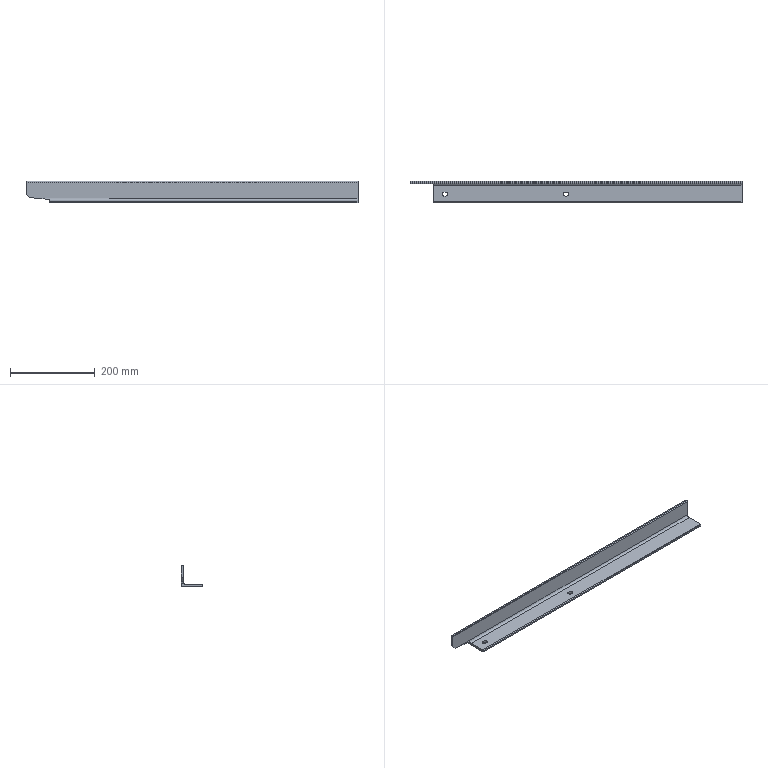Part | SolidWorks | 1 solid | 25 faces | box 783.5 x 50 x 50 mm | volume 359251 mm3 | plane 16 | cylinder 9 | commonest cylinder face diameters 9 x6 3.333 x2 11 x1
STEP:
#1=CARTESIAN_POINT('',(-21.75,-25.5,0.));
#2=VERTEX_POINT('',#1);
#3=CARTESIAN_POINT('',(-17.25,-30.,0.));
#4=VERTEX_POINT('',#3);
#5=CARTESIAN_POINT('',(-21.75,-30.,0.));
#6=DIRECTION('',(0.,0.,-1.));
#7=DIRECTION('',(1.,0.,0.));
#8=AXIS2_PLACEMENT_3D('',#5,#6,#7);
#9=CIRCLE('',#8,4.5);
#10=EDGE_CURVE('',#2,#4,#9,.T.);
#11=ORIENTED_EDGE('',*,*,#10,.T.);
#12=CARTESIAN_POINT('',(-17.25,-30.,5.));
#13=VERTEX_POINT('',#12);
#14=CARTESIAN_POINT('',(-17.25,-30.,-0.001));
#15=DIRECTION('',(0.,0.,1.));
#16=VECTOR('',#15,1000.);
#17=LINE('',#14,#16);
#18=EDGE_CURVE('',#4,#13,#17,.T.);
#19=ORIENTED_EDGE('',*,*,#18,.T.);
#20=CARTESIAN_POINT('',(-21.75,-25.5,5.));
#21=VERTEX_POINT('',#20);
#22=CARTESIAN_POINT('',(-21.75,-30.,5.));
#23=DIRECTION('',(0.,0.,1.));
#24=DIRECTION('',(1.,0.,0.));
#25=AXIS2_PLACEMENT_3D('',#22,#23,#24);
#26=CIRCLE('',#25,4.5);
#27=EDGE_CURVE('',#13,#21,#26,.T.);
#28=ORIENTED_EDGE('',*,*,#27,.T.);
#29=CARTESIAN_POINT('',(-21.75,-25.5,-0.001));
#30=DIRECTION('',(0.,0.,1.));
#31=VECTOR('',#30,1000.);
#32=LINE('',#29,#31);
#33=EDGE_CURVE('',#2,#21,#32,.T.);
#34=ORIENTED_EDGE('',*,*,#33,.F.);
#35=EDGE_LOOP('',(#11,#19,#28,#34));
#36=FACE_OUTER_BOUND('',#35,.T.);
#37=CARTESIAN_POINT('',(-21.75,-30.,-0.001));
#38=DIRECTION('',(0.,0.,1.));
#39=DIRECTION('',(1.,0.,0.));
#40=AXIS2_PLACEMENT_3D('',#37,#38,#39);
#41=CYLINDRICAL_SURFACE('',#40,4.5);
#42=ADVANCED_FACE('',(#36),#41,.F.);
#43=CARTESIAN_POINT('',(-307.75,-25.5,0.));
#44=VERTEX_POINT('',#43);
#45=CARTESIAN_POINT('',(-303.25,-30.,0.));
#46=VERTEX_POINT('',#45);
#47=CARTESIAN_POINT('',(-307.75,-30.,0.));
#48=DIRECTION('',(0.,0.,-1.));
#49=DIRECTION('',(1.,0.,0.));
#50=AXIS2_PLACEMENT_3D('',#47,#48,#49);
#51=CIRCLE('',#50,4.5);
#52=EDGE_CURVE('',#44,#46,#51,.T.);
#53=ORIENTED_EDGE('',*,*,#52,.T.);
#54=CARTESIAN_POINT('',(-303.25,-30.,5.));
#55=VERTEX_POINT('',#54);
#56=CARTESIAN_POINT('',(-303.25,-30.,-0.001));
#57=DIRECTION('',(0.,0.,1.));
#58=VECTOR('',#57,1000.);
#59=LINE('',#56,#58);
#60=EDGE_CURVE('',#46,#55,#59,.T.);
#61=ORIENTED_EDGE('',*,*,#60,.T.);
#62=CARTESIAN_POINT('',(-307.75,-25.5,5.));
#63=VERTEX_POINT('',#62);
#64=CARTESIAN_POINT('',(-307.75,-30.,5.));
#65=DIRECTION('',(0.,0.,1.));
#66=DIRECTION('',(1.,0.,0.));
#67=AXIS2_PLACEMENT_3D('',#64,#65,#66);
#68=CIRCLE('',#67,4.5);
#69=EDGE_CURVE('',#55,#63,#68,.T.);
#70=ORIENTED_EDGE('',*,*,#69,.T.);
#71=CARTESIAN_POINT('',(-307.75,-25.5,-0.001));
#72=DIRECTION('',(0.,0.,1.));
#73=VECTOR('',#72,1000.);
#74=LINE('',#71,#73);
#75=EDGE_CURVE('',#44,#63,#74,.T.);
#76=ORIENTED_EDGE('',*,*,#75,.F.);
#77=EDGE_LOOP('',(#53,#61,#70,#76));
#78=FACE_OUTER_BOUND('',#77,.T.);
#79=CARTESIAN_POINT('',(-307.75,-30.,-0.001));
#80=DIRECTION('',(0.,0.,1.));
#81=DIRECTION('',(1.,0.,0.));
#82=AXIS2_PLACEMENT_3D('',#79,#80,#81);
#83=CYLINDRICAL_SURFACE('',#82,4.5);
#84=ADVANCED_FACE('',(#78),#83,.F.);
#85=CARTESIAN_POINT('',(-25.75,-25.5,0.));
#86=VERTEX_POINT('',#85);
#87=CARTESIAN_POINT('',(-25.75,-25.5,0.));
#88=DIRECTION('',(1.,0.,0.));
#89=VECTOR('',#88,1000.);
#90=LINE('',#87,#89);
#91=EDGE_CURVE('',#86,#2,#90,.T.);
#92=ORIENTED_EDGE('',*,*,#91,.F.);
#93=CARTESIAN_POINT('',(-25.75,-34.5,0.));
#94=VERTEX_POINT('',#93);
#95=CARTESIAN_POINT('',(-25.75,-30.,0.));
#96=DIRECTION('',(0.,0.,-1.));
#97=DIRECTION('',(1.,0.,0.));
#98=AXIS2_PLACEMENT_3D('',#95,#96,#97);
#99=CIRCLE('',#98,4.5);
#100=EDGE_CURVE('',#94,#86,#99,.T.);
#101=ORIENTED_EDGE('',*,*,#100,.F.);
#102=CARTESIAN_POINT('',(-21.75,-34.5,0.));
#103=VERTEX_POINT('',#102);
#104=CARTESIAN_POINT('',(-25.75,-34.5,0.));
#105=DIRECTION('',(-1.,0.,0.));
#106=VECTOR('',#105,1000.);
#107=LINE('',#104,#106);
#108=EDGE_CURVE('',#103,#94,#107,.T.);
#109=ORIENTED_EDGE('',*,*,#108,.F.);
#110=CARTESIAN_POINT('',(-21.75,-30.,0.));
#111=DIRECTION('',(0.,0.,-1.));
#112=DIRECTION('',(1.,0.,0.));
#113=AXIS2_PLACEMENT_3D('',#110,#111,#112);
#114=CIRCLE('',#113,4.5);
#115=EDGE_CURVE('',#4,#103,#114,.T.);
#116=ORIENTED_EDGE('',*,*,#115,.F.);
#117=ORIENTED_EDGE('',*,*,#10,.F.);
#118=EDGE_LOOP('',(#92,#101,#109,#116,#117));
#119=FACE_BOUND('',#118,.T.);
#120=CARTESIAN_POINT('',(-311.75,-25.5,0.));
#121=VERTEX_POINT('',#120);
#122=CARTESIAN_POINT('',(-311.75,-25.5,0.));
#123=DIRECTION('',(1.,0.,0.));
#124=VECTOR('',#123,1000.);
#125=LINE('',#122,#124);
#126=EDGE_CURVE('',#121,#44,#125,.T.);
#127=ORIENTED_EDGE('',*,*,#126,.F.);
#128=CARTESIAN_POINT('',(-311.75,-34.5,0.));
#129=VERTEX_POINT('',#128);
#130=CARTESIAN_POINT('',(-311.75,-30.,0.));
#131=DIRECTION('',(0.,0.,-1.));
#132=DIRECTION('',(1.,0.,0.));
#133=AXIS2_PLACEMENT_3D('',#130,#131,#132);
#134=CIRCLE('',#133,4.5);
#135=EDGE_CURVE('',#129,#121,#134,.T.);
#136=ORIENTED_EDGE('',*,*,#135,.F.);
#137=CARTESIAN_POINT('',(-307.75,-34.5,0.));
#138=VERTEX_POINT('',#137);
#139=CARTESIAN_POINT('',(-311.75,-34.5,0.));
#140=DIRECTION('',(-1.,0.,0.));
#141=VECTOR('',#140,1000.);
#142=LINE('',#139,#141);
#143=EDGE_CURVE('',#138,#129,#142,.T.);
#144=ORIENTED_EDGE('',*,*,#143,.F.);
#145=CARTESIAN_POINT('',(-307.75,-30.,0.));
#146=DIRECTION('',(0.,0.,-1.));
#147=DIRECTION('',(1.,0.,0.));
#148=AXIS2_PLACEMENT_3D('',#145,#146,#147);
#149=CIRCLE('',#148,4.5);
#150=EDGE_CURVE('',#46,#138,#149,.T.);
#151=ORIENTED_EDGE('',*,*,#150,.F.);
#152=ORIENTED_EDGE('',*,*,#52,.F.);
#153=EDGE_LOOP('',(#127,#136,#144,#151,#152));
#154=FACE_BOUND('',#153,.T.);
#155=CARTESIAN_POINT('',(-335.25,-50.,0.));
#156=VERTEX_POINT('',#155);
#157=CARTESIAN_POINT('',(391.75,-50.,0.));
#158=VERTEX_POINT('',#157);
#159=CARTESIAN_POINT('',(-391.75,-50.,0.));
#160=DIRECTION('',(1.,0.,0.));
#161=VECTOR('',#160,1000.);
#162=LINE('',#159,#161);
#163=EDGE_CURVE('',#156,#158,#162,.T.);
#164=ORIENTED_EDGE('',*,*,#163,.F.);
#165=CARTESIAN_POINT('',(-335.25,0.,0.));
#166=VERTEX_POINT('',#165);
#167=CARTESIAN_POINT('',(-335.25,-50.,0.));
#168=DIRECTION('',(0.,1.,0.));
#169=VECTOR('',#168,1000.);
#170=LINE('',#167,#169);
#171=EDGE_CURVE('',#156,#166,#170,.T.);
#172=ORIENTED_EDGE('',*,*,#171,.T.);
#173=CARTESIAN_POINT('',(391.75,0.,0.));
#174=VERTEX_POINT('',#173);
#175=CARTESIAN_POINT('',(-391.75,0.,0.));
#176=DIRECTION('',(1.,0.,0.));
#177=VECTOR('',#176,1000.);
#178=LINE('',#175,#177);
#179=EDGE_CURVE('',#166,#174,#178,.T.);
#180=ORIENTED_EDGE('',*,*,#179,.T.);
#181=CARTESIAN_POINT('',(391.75,-50.,0.));
#182=DIRECTION('',(0.,-1.,0.));
#183=VECTOR('',#182,1000.);
#184=LINE('',#181,#183);
#185=EDGE_CURVE('',#174,#158,#184,.T.);
#186=ORIENTED_EDGE('',*,*,#185,.T.);
#187=EDGE_LOOP('',(#164,#172,#180,#186));
#188=FACE_OUTER_BOUND('',#187,.T.);
#189=CARTESIAN_POINT('',(-391.75,-50.,0.));
#190=DIRECTION('',(0.,0.,1.));
#191=DIRECTION('',(1.,0.,0.));
#192=AXIS2_PLACEMENT_3D('',#189,#190,#191);
#193=PLANE('',#192);
#194=ADVANCED_FACE('',(#119,#154,#188),#193,.F.);
#195=CARTESIAN_POINT('',(-335.25,-50.,3.333));
#196=VERTEX_POINT('',#195);
#197=CARTESIAN_POINT('',(391.75,-50.,3.333));
#198=VERTEX_POINT('',#197);
#199=CARTESIAN_POINT('',(-391.75,-50.,3.333));
#200=DIRECTION('',(1.,0.,0.));
#201=VECTOR('',#200,1000.);
#202=LINE('',#199,#201);
#203=EDGE_CURVE('',#196,#198,#202,.T.);
#204=ORIENTED_EDGE('',*,*,#203,.F.);
#205=CARTESIAN_POINT('',(-335.25,-50.,-7.499));
#206=DIRECTION('',(0.,0.,-1.));
#207=VECTOR('',#206,1000.);
#208=LINE('',#205,#207);
#209=EDGE_CURVE('',#196,#156,#208,.T.);
#210=ORIENTED_EDGE('',*,*,#209,.T.);
#211=ORIENTED_EDGE('',*,*,#163,.T.);
#212=CARTESIAN_POINT('',(391.75,-50.,0.));
#213=DIRECTION('',(0.,0.,1.));
#214=VECTOR('',#213,1000.);
#215=LINE('',#212,#214);
#216=EDGE_CURVE('',#158,#198,#215,.T.);
#217=ORIENTED_EDGE('',*,*,#216,.T.);
#218=EDGE_LOOP('',(#204,#210,#211,#217));
#219=FACE_OUTER_BOUND('',#218,.T.);
#220=CARTESIAN_POINT('',(-391.75,-50.,0.));
#221=DIRECTION('',(0.,1.,0.));
#222=DIRECTION('',(-1.,0.,0.));
#223=AXIS2_PLACEMENT_3D('',#220,#221,#222);
#224=PLANE('',#223);
#225=ADVANCED_FACE('',(#219),#224,.F.);
#226=CARTESIAN_POINT('',(-335.25,-48.333,5.));
#227=VERTEX_POINT('',#226);
#228=CARTESIAN_POINT('',(391.75,-48.333,5.));
#229=VERTEX_POINT('',#228);
#230=CARTESIAN_POINT('',(-391.75,-48.333,5.));
#231=DIRECTION('',(1.,0.,0.));
#232=VECTOR('',#231,1000.);
#233=LINE('',#230,#232);
#234=EDGE_CURVE('',#227,#229,#233,.T.);
#235=ORIENTED_EDGE('',*,*,#234,.F.);
#236=CARTESIAN_POINT('',(-335.25,-48.333,3.333));
#237=DIRECTION('',(1.,0.,0.));
#238=DIRECTION('',(0.,0.,-1.));
#239=AXIS2_PLACEMENT_3D('',#236,#237,#238);
#240=CIRCLE('',#239,1.667);
#241=EDGE_CURVE('',#227,#196,#240,.T.);
#242=ORIENTED_EDGE('',*,*,#241,.T.);
#243=ORIENTED_EDGE('',*,*,#203,.T.);
#244=CARTESIAN_POINT('',(391.75,-48.333,3.333));
#245=DIRECTION('',(-1.,0.,0.));
#246=DIRECTION('',(0.,-1.,0.));
#247=AXIS2_PLACEMENT_3D('',#244,#245,#246);
#248=CIRCLE('',#247,1.667);
#249=EDGE_CURVE('',#198,#229,#248,.T.);
#250=ORIENTED_EDGE('',*,*,#249,.T.);
#251=EDGE_LOOP('',(#235,#242,#243,#250));
#252=FACE_OUTER_BOUND('',#251,.T.);
#253=CARTESIAN_POINT('',(-391.75,-48.333,3.333));
#254=DIRECTION('',(1.,0.,0.));
#255=DIRECTION('',(0.,1.,0.));
#256=AXIS2_PLACEMENT_3D('',#253,#254,#255);
#257=CYLINDRICAL_SURFACE('',#256,1.667);
#258=ADVANCED_FACE('',(#252),#257,.T.);
#259=CARTESIAN_POINT('',(-25.75,-34.5,5.));
#260=VERTEX_POINT('',#259);
#261=CARTESIAN_POINT('',(-21.75,-34.5,5.));
#262=VERTEX_POINT('',#261);
#263=CARTESIAN_POINT('',(-25.75,-34.5,5.));
#264=DIRECTION('',(1.,0.,0.));
#265=VECTOR('',#264,1000.);
#266=LINE('',#263,#265);
#267=EDGE_CURVE('',#260,#262,#266,.T.);
#268=ORIENTED_EDGE('',*,*,#267,.F.);
#269=CARTESIAN_POINT('',(-25.75,-25.5,5.));
#270=VERTEX_POINT('',#269);
#271=CARTESIAN_POINT('',(-25.75,-30.,5.));
#272=DIRECTION('',(0.,0.,1.));
#273=DIRECTION('',(1.,0.,0.));
#274=AXIS2_PLACEMENT_3D('',#271,#272,#273);
#275=CIRCLE('',#274,4.5);
#276=EDGE_CURVE('',#270,#260,#275,.T.);
#277=ORIENTED_EDGE('',*,*,#276,.F.);
#278=CARTESIAN_POINT('',(-25.75,-25.5,5.));
#279=DIRECTION('',(-1.,0.,0.));
#280=VECTOR('',#279,1000.);
#281=LINE('',#278,#280);
#282=EDGE_CURVE('',#21,#270,#281,.T.);
#283=ORIENTED_EDGE('',*,*,#282,.F.);
#284=ORIENTED_EDGE('',*,*,#27,.F.);
#285=CARTESIAN_POINT('',(-21.75,-30.,5.));
#286=DIRECTION('',(0.,0.,1.));
#287=DIRECTION('',(1.,0.,0.));
#288=AXIS2_PLACEMENT_3D('',#285,#286,#287);
#289=CIRCLE('',#288,4.5);
#290=EDGE_CURVE('',#262,#13,#289,.T.);
#291=ORIENTED_EDGE('',*,*,#290,.F.);
#292=EDGE_LOOP('',(#268,#277,#283,#284,#291));
#293=FACE_BOUND('',#292,.T.);
#294=CARTESIAN_POINT('',(-311.75,-34.5,5.));
#295=VERTEX_POINT('',#294);
#296=CARTESIAN_POINT('',(-307.75,-34.5,5.));
#297=VERTEX_POINT('',#296);
#298=CARTESIAN_POINT('',(-311.75,-34.5,5.));
#299=DIRECTION('',(1.,0.,0.));
#300=VECTOR('',#299,1000.);
#301=LINE('',#298,#300);
#302=EDGE_CURVE('',#295,#297,#301,.T.);
#303=ORIENTED_EDGE('',*,*,#302,.F.);
#304=CARTESIAN_POINT('',(-311.75,-25.5,5.));
#305=VERTEX_POINT('',#304);
#306=CARTESIAN_POINT('',(-311.75,-30.,5.));
#307=DIRECTION('',(0.,0.,1.));
#308=DIRECTION('',(1.,0.,0.));
#309=AXIS2_PLACEMENT_3D('',#306,#307,#308);
#310=CIRCLE('',#309,4.5);
#311=EDGE_CURVE('',#305,#295,#310,.T.);
#312=ORIENTED_EDGE('',*,*,#311,.F.);
#313=CARTESIAN_POINT('',(-311.75,-25.5,5.));
#314=DIRECTION('',(-1.,0.,0.));
#315=VECTOR('',#314,1000.);
#316=LINE('',#313,#315);
#317=EDGE_CURVE('',#63,#305,#316,.T.);
#318=ORIENTED_EDGE('',*,*,#317,.F.);
#319=ORIENTED_EDGE('',*,*,#69,.F.);
#320=CARTESIAN_POINT('',(-307.75,-30.,5.));
#321=DIRECTION('',(0.,0.,1.));
#322=DIRECTION('',(1.,0.,0.));
#323=AXIS2_PLACEMENT_3D('',#320,#321,#322);
#324=CIRCLE('',#323,4.5);
#325=EDGE_CURVE('',#297,#55,#324,.T.);
#326=ORIENTED_EDGE('',*,*,#325,.F.);
#327=EDGE_LOOP('',(#303,#312,#318,#319,#326));
#328=FACE_BOUND('',#327,.T.);
#329=CARTESIAN_POINT('',(-335.25,-10.5,5.));
#330=VERTEX_POINT('',#329);
#331=CARTESIAN_POINT('',(391.75,-10.5,5.));
#332=VERTEX_POINT('',#331);
#333=CARTESIAN_POINT('',(-391.75,-10.5,5.));
#334=DIRECTION('',(1.,0.,0.));
#335=VECTOR('',#334,1000.);
#336=LINE('',#333,#335);
#337=EDGE_CURVE('',#330,#332,#336,.T.);
#338=ORIENTED_EDGE('',*,*,#337,.F.);
#339=CARTESIAN_POINT('',(-335.25,-10.5,5.));
#340=DIRECTION('',(0.,-1.,0.));
#341=VECTOR('',#340,1000.);
#342=LINE('',#339,#341);
#343=EDGE_CURVE('',#330,#227,#342,.T.);
#344=ORIENTED_EDGE('',*,*,#343,.T.);
#345=ORIENTED_EDGE('',*,*,#234,.T.);
#346=CARTESIAN_POINT('',(391.75,-10.5,5.));
#347=DIRECTION('',(0.,1.,0.));
#348=VECTOR('',#347,1000.);
#349=LINE('',#346,#348);
#350=EDGE_CURVE('',#229,#332,#349,.T.);
#351=ORIENTED_EDGE('',*,*,#350,.T.);
#352=EDGE_LOOP('',(#338,#344,#345,#351));
#353=FACE_OUTER_BOUND('',#352,.T.);
#354=CARTESIAN_POINT('',(-391.75,-10.5,5.));
#355=DIRECTION('',(0.,0.,-1.));
#356=DIRECTION('',(0.,1.,0.));
#357=AXIS2_PLACEMENT_3D('',#354,#355,#356);
#358=PLANE('',#357);
#359=ADVANCED_FACE('',(#293,#328,#353),#358,.F.);
#360=CARTESIAN_POINT('',(-339.727,-5.889,7.501));
#361=VERTEX_POINT('',#360);
#362=CARTESIAN_POINT('',(-335.25,-5.889,7.501));
#363=VERTEX_POINT('',#362);
#364=CARTESIAN_POINT('',(-391.75,-5.889,7.501));
#365=DIRECTION('',(1.,0.,0.));
#366=VECTOR('',#365,1000.);
#367=LINE('',#364,#366);
#368=EDGE_CURVE('',#361,#363,#367,.T.);
#369=ORIENTED_EDGE('',*,*,#368,.T.);
#370=CARTESIAN_POINT('',(-335.25,-10.5,10.5));
#371=DIRECTION('',(-1.,0.,0.));
#372=DIRECTION('',(0.,0.,-1.));
#373=AXIS2_PLACEMENT_3D('',#370,#371,#372);
#374=CIRCLE('',#373,5.5);
#375=EDGE_CURVE('',#363,#330,#374,.T.);
#376=ORIENTED_EDGE('',*,*,#375,.T.);
#377=ORIENTED_EDGE('',*,*,#337,.T.);
#378=CARTESIAN_POINT('',(391.75,-5.,10.5));
#379=VERTEX_POINT('',#378);
#380=CARTESIAN_POINT('',(391.75,-10.5,10.5));
#381=DIRECTION('',(1.,0.,0.));
#382=DIRECTION('',(0.,1.,0.));
#383=AXIS2_PLACEMENT_3D('',#380,#381,#382);
#384=CIRCLE('',#383,5.5);
#385=EDGE_CURVE('',#332,#379,#384,.T.);
#386=ORIENTED_EDGE('',*,*,#385,.T.);
#387=CARTESIAN_POINT('',(-368.257,-5.,10.5));
#388=VERTEX_POINT('',#387);
#389=CARTESIAN_POINT('',(-391.75,-5.,10.5));
#390=DIRECTION('',(1.,0.,0.));
#391=VECTOR('',#390,1000.);
#392=LINE('',#389,#391);
#393=EDGE_CURVE('',#388,#379,#392,.T.);
#394=ORIENTED_EDGE('',*,*,#393,.F.);
#395=CARTESIAN_POINT('',(-368.257,-5.,10.5));
#396=CARTESIAN_POINT('',(-358.057,-5.,9.428));
#397=CARTESIAN_POINT('',(-348.278,-5.305,8.4));
#398=CARTESIAN_POINT('',(-339.727,-5.889,7.501));
#399=(BOUNDED_CURVE()B_SPLINE_CURVE(3,(#395,#396,#397,#398),.UNSPECIFIED.,.F.,.F.)B_SPLINE_CURVE_WITH_KNOTS((4,4),(4.712,5.289),.UNSPECIFIED.)CURVE()GEOMETRIC_REPRESENTATION_ITEM()RATIONAL_B_SPLINE_CURVE((1.,0.9725,0.9725,1.))REPRESENTATION_ITEM(''));
#400=EDGE_CURVE('',#388,#361,#399,.T.);
#401=ORIENTED_EDGE('',*,*,#400,.T.);
#402=EDGE_LOOP('',(#369,#376,#377,#386,#394,#401));
#403=FACE_OUTER_BOUND('',#402,.T.);
#404=CARTESIAN_POINT('',(-391.75,-10.5,10.5));
#405=DIRECTION('',(1.,0.,0.));
#406=DIRECTION('',(0.,1.,0.));
#407=AXIS2_PLACEMENT_3D('',#404,#405,#406);
#408=CYLINDRICAL_SURFACE('',#407,5.5);
#409=ADVANCED_FACE('',(#403),#408,.F.);
#410=CARTESIAN_POINT('',(-391.75,-5.,21.973));
#411=VERTEX_POINT('',#410);
#412=CARTESIAN_POINT('',(-382.795,-5.,12.028));
#413=VERTEX_POINT('',#412);
#414=CARTESIAN_POINT('',(-404.858,-5.,36.531));
#415=DIRECTION('',(0.6691,0.,-0.7431));
#416=VECTOR('',#415,1000.);
#417=LINE('',#414,#416);
#418=EDGE_CURVE('',#411,#413,#417,.T.);
#419=ORIENTED_EDGE('',*,*,#418,.T.);
#420=CARTESIAN_POINT('',(-395.426,-5.,13.356));
#421=DIRECTION('',(0.9945,0.,-0.1045));
#422=VECTOR('',#421,1000.);
#423=LINE('',#420,#422);
#424=EDGE_CURVE('',#413,#388,#423,.T.);
#425=ORIENTED_EDGE('',*,*,#424,.T.);
#426=ORIENTED_EDGE('',*,*,#393,.T.);
#427=CARTESIAN_POINT('',(391.75,-5.,48.333));
#428=VERTEX_POINT('',#427);
#429=CARTESIAN_POINT('',(391.75,-5.,48.333));
#430=DIRECTION('',(0.,0.,1.));
#431=VECTOR('',#430,1000.);
#432=LINE('',#429,#431);
#433=EDGE_CURVE('',#379,#428,#432,.T.);
#434=ORIENTED_EDGE('',*,*,#433,.T.);
#435=CARTESIAN_POINT('',(-391.75,-5.,48.333));
#436=VERTEX_POINT('',#435);
#437=CARTESIAN_POINT('',(-391.75,-5.,48.333));
#438=DIRECTION('',(1.,0.,0.));
#439=VECTOR('',#438,1000.);
#440=LINE('',#437,#439);
#441=EDGE_CURVE('',#436,#428,#440,.T.);
#442=ORIENTED_EDGE('',*,*,#441,.F.);
#443=CARTESIAN_POINT('',(-391.75,-5.,48.333));
#444=DIRECTION('',(0.,0.,1.));
#445=VECTOR('',#444,1000.);
#446=LINE('',#443,#445);
#447=EDGE_CURVE('',#411,#436,#446,.T.);
#448=ORIENTED_EDGE('',*,*,#447,.F.);
#449=EDGE_LOOP('',(#419,#425,#426,#434,#442,#448));
#450=FACE_OUTER_BOUND('',#449,.T.);
#451=CARTESIAN_POINT('',(-391.75,-5.,48.333));
#452=DIRECTION('',(0.,1.,0.));
#453=DIRECTION('',(-1.,0.,0.));
#454=AXIS2_PLACEMENT_3D('',#451,#452,#453);
#455=PLANE('',#454);
#456=ADVANCED_FACE('',(#450),#455,.F.);
#457=CARTESIAN_POINT('',(391.75,-3.333,50.));
#458=VERTEX_POINT('',#457);
#459=CARTESIAN_POINT('',(391.75,-3.333,48.333));
#460=DIRECTION('',(-1.,0.,0.));
#461=DIRECTION('',(0.,1.,0.));
#462=AXIS2_PLACEMENT_3D('',#459,#460,#461);
#463=CIRCLE('',#462,1.667);
#464=EDGE_CURVE('',#428,#458,#463,.T.);
#465=ORIENTED_EDGE('',*,*,#464,.T.);
#466=CARTESIAN_POINT('',(-391.75,-3.333,50.));
#467=VERTEX_POINT('',#466);
#468=CARTESIAN_POINT('',(-391.75,-3.333,50.));
#469=DIRECTION('',(1.,0.,0.));
#470=VECTOR('',#469,1000.);
#471=LINE('',#468,#470);
#472=EDGE_CURVE('',#467,#458,#471,.T.);
#473=ORIENTED_EDGE('',*,*,#472,.F.);
#474=CARTESIAN_POINT('',(-391.75,-3.333,48.333));
#475=DIRECTION('',(-1.,0.,0.));
#476=DIRECTION('',(0.,1.,0.));
#477=AXIS2_PLACEMENT_3D('',#474,#475,#476);
#478=CIRCLE('',#477,1.667);
#479=EDGE_CURVE('',#436,#467,#478,.T.);
#480=ORIENTED_EDGE('',*,*,#479,.F.);
#481=ORIENTED_EDGE('',*,*,#441,.T.);
#482=EDGE_LOOP('',(#465,#473,#480,#481));
#483=FACE_OUTER_BOUND('',#482,.T.);
#484=CARTESIAN_POINT('',(-391.75,-3.333,48.333));
#485=DIRECTION('',(1.,0.,0.));
#486=DIRECTION('',(0.,1.,0.));
#487=AXIS2_PLACEMENT_3D('',#484,#485,#486);
#488=CYLINDRICAL_SURFACE('',#487,1.667);
#489=ADVANCED_FACE('',(#483),#488,.T.);
#490=CARTESIAN_POINT('',(391.75,0.,50.));
#491=VERTEX_POINT('',#490);
#492=CARTESIAN_POINT('',(391.75,0.,50.));
#493=DIRECTION('',(0.,1.,0.));
#494=VECTOR('',#493,1000.);
#495=LINE('',#492,#494);
#496=EDGE_CURVE('',#458,#491,#495,.T.);
#497=ORIENTED_EDGE('',*,*,#496,.T.);
#498=CARTESIAN_POINT('',(-391.75,0.,50.));
#499=VERTEX_POINT('',#498);
#500=CARTESIAN_POINT('',(-391.75,0.,50.));
#501=DIRECTION('',(1.,0.,0.));
#502=VECTOR('',#501,1000.);
#503=LINE('',#500,#502);
#504=EDGE_CURVE('',#499,#491,#503,.T.);
#505=ORIENTED_EDGE('',*,*,#504,.F.);
#506=CARTESIAN_POINT('',(-391.75,0.,50.));
#507=DIRECTION('',(0.,1.,0.));
#508=VECTOR('',#507,1000.);
#509=LINE('',#506,#508);
#510=EDGE_CURVE('',#467,#499,#509,.T.);
#511=ORIENTED_EDGE('',*,*,#510,.F.);
#512=ORIENTED_EDGE('',*,*,#472,.T.);
#513=EDGE_LOOP('',(#497,#505,#511,#512));
#514=FACE_OUTER_BOUND('',#513,.T.);
#515=CARTESIAN_POINT('',(-391.75,0.,50.));
#516=DIRECTION('',(0.,0.,-1.));
#517=DIRECTION('',(0.,1.,0.));
#518=AXIS2_PLACEMENT_3D('',#515,#516,#517);
#519=PLANE('',#518);
#520=ADVANCED_FACE('',(#514),#519,.F.);
#521=ORIENTED_EDGE('',*,*,#179,.F.);
#522=CARTESIAN_POINT('',(-335.25,0.,7.501));
#523=VERTEX_POINT('',#522);
#524=CARTESIAN_POINT('',(-335.25,0.,0.));
#525=DIRECTION('',(0.,0.,-1.));
#526=VECTOR('',#525,1000.);
#527=LINE('',#524,#526);
#528=EDGE_CURVE('',#523,#166,#527,.T.);
#529=ORIENTED_EDGE('',*,*,#528,.F.);
#530=CARTESIAN_POINT('',(-339.727,0.,7.501));
#531=VERTEX_POINT('',#530);
#532=CARTESIAN_POINT('',(-335.25,0.,7.501));
#533=DIRECTION('',(1.,0.,0.));
#534=VECTOR('',#533,1000.);
#535=LINE('',#532,#534);
#536=EDGE_CURVE('',#531,#523,#535,.T.);
#537=ORIENTED_EDGE('',*,*,#536,.F.);
#538=CARTESIAN_POINT('',(-382.795,0.,12.028));
#539=VERTEX_POINT('',#538);
#540=CARTESIAN_POINT('',(-339.727,0.,7.501));
#541=DIRECTION('',(0.9945,0.,-0.1045));
#542=VECTOR('',#541,1000.);
#543=LINE('',#540,#542);
#544=EDGE_CURVE('',#539,#531,#543,.T.);
#545=ORIENTED_EDGE('',*,*,#544,.F.);
#546=CARTESIAN_POINT('',(-391.75,0.,21.973));
#547=VERTEX_POINT('',#546);
#548=CARTESIAN_POINT('',(-382.795,0.,12.028));
#549=DIRECTION('',(0.6691,0.,-0.7431));
#550=VECTOR('',#549,1000.);
#551=LINE('',#548,#550);
#552=EDGE_CURVE('',#547,#539,#551,.T.);
#553=ORIENTED_EDGE('',*,*,#552,.F.);
#554=CARTESIAN_POINT('',(-391.75,0.,0.));
#555=DIRECTION('',(0.,0.,-1.));
#556=VECTOR('',#555,1000.);
#557=LINE('',#554,#556);
#558=EDGE_CURVE('',#499,#547,#557,.T.);
#559=ORIENTED_EDGE('',*,*,#558,.F.);
#560=ORIENTED_EDGE('',*,*,#504,.T.);
#561=CARTESIAN_POINT('',(391.75,0.,0.));
#562=DIRECTION('',(0.,0.,-1.));
#563=VECTOR('',#562,1000.);
#564=LINE('',#561,#563);
#565=EDGE_CURVE('',#491,#174,#564,.T.);
#566=ORIENTED_EDGE('',*,*,#565,.T.);
#567=EDGE_LOOP('',(#521,#529,#537,#545,#553,#559,#560,#566));
#568=FACE_OUTER_BOUND('',#567,.T.);
#569=CARTESIAN_POINT('',(-391.75,0.,0.));
#570=DIRECTION('',(0.,-1.,0.));
#571=DIRECTION('',(1.,0.,0.));
#572=AXIS2_PLACEMENT_3D('',#569,#570,#571);
#573=PLANE('',#572);
#574=ADVANCED_FACE('',(#568),#573,.F.);
#575=ORIENTED_EDGE('',*,*,#558,.T.);
#576=CARTESIAN_POINT('',(-391.75,-3.333,21.973));
#577=DIRECTION('',(0.,-1.,0.));
#578=VECTOR('',#577,1000.);
#579=LINE('',#576,#578);
#580=EDGE_CURVE('',#547,#411,#579,.T.);
#581=ORIENTED_EDGE('',*,*,#580,.T.);
#582=ORIENTED_EDGE('',*,*,#447,.T.);
#583=ORIENTED_EDGE('',*,*,#479,.T.);
#584=ORIENTED_EDGE('',*,*,#510,.T.);
#585=EDGE_LOOP('',(#575,#581,#582,#583,#584));
#586=FACE_OUTER_BOUND('',#585,.T.);
#587=CARTESIAN_POINT('',(-391.75,-3.333,48.333));
#588=DIRECTION('',(1.,0.,0.));
#589=DIRECTION('',(0.,1.,0.));
#590=AXIS2_PLACEMENT_3D('',#587,#588,#589);
#591=PLANE('',#590);
#592=ADVANCED_FACE('',(#586),#591,.F.);
#593=ORIENTED_EDGE('',*,*,#185,.F.);
#594=ORIENTED_EDGE('',*,*,#565,.F.);
#595=ORIENTED_EDGE('',*,*,#496,.F.);
#596=ORIENTED_EDGE('',*,*,#464,.F.);
#597=ORIENTED_EDGE('',*,*,#433,.F.);
#598=ORIENTED_EDGE('',*,*,#385,.F.);
#599=ORIENTED_EDGE('',*,*,#350,.F.);
#600=ORIENTED_EDGE('',*,*,#249,.F.);
#601=ORIENTED_EDGE('',*,*,#216,.F.);
#602=EDGE_LOOP('',(#593,#594,#595,#596,#597,#598,#599,#600,#601));
#603=FACE_OUTER_BOUND('',#602,.T.);
#604=CARTESIAN_POINT('',(391.75,-3.333,48.333));
#605=DIRECTION('',(1.,0.,0.));
#606=DIRECTION('',(0.,1.,0.));
#607=AXIS2_PLACEMENT_3D('',#604,#605,#606);
#608=PLANE('',#607);
#609=ADVANCED_FACE('',(#603),#608,.T.);
#610=ORIENTED_EDGE('',*,*,#209,.F.);
#611=ORIENTED_EDGE('',*,*,#241,.F.);
#612=ORIENTED_EDGE('',*,*,#343,.F.);
#613=ORIENTED_EDGE('',*,*,#375,.F.);
#614=CARTESIAN_POINT('',(-335.25,-50.,7.501));
#615=DIRECTION('',(0.,1.,0.));
#616=VECTOR('',#615,1000.);
#617=LINE('',#614,#616);
#618=EDGE_CURVE('',#363,#523,#617,.T.);
#619=ORIENTED_EDGE('',*,*,#618,.T.);
#620=ORIENTED_EDGE('',*,*,#528,.T.);
#621=ORIENTED_EDGE('',*,*,#171,.F.);
#622=EDGE_LOOP('',(#610,#611,#612,#613,#619,#620,#621));
#623=FACE_OUTER_BOUND('',#622,.T.);
#624=CARTESIAN_POINT('',(-335.25,-50.,0.));
#625=DIRECTION('',(1.,0.,0.));
#626=DIRECTION('',(0.,0.,-1.));
#627=AXIS2_PLACEMENT_3D('',#624,#625,#626);
#628=PLANE('',#627);
#629=ADVANCED_FACE('',(#623),#628,.F.);
#630=CARTESIAN_POINT('',(-339.727,-50.,7.501));
#631=DIRECTION('',(0.,1.,0.));
#632=VECTOR('',#631,1000.);
#633=LINE('',#630,#632);
#634=EDGE_CURVE('',#361,#531,#633,.T.);
#635=ORIENTED_EDGE('',*,*,#634,.T.);
#636=ORIENTED_EDGE('',*,*,#536,.T.);
#637=ORIENTED_EDGE('',*,*,#618,.F.);
#638=ORIENTED_EDGE('',*,*,#368,.F.);
#639=EDGE_LOOP('',(#635,#636,#637,#638));
#640=FACE_OUTER_BOUND('',#639,.T.);
#641=CARTESIAN_POINT('',(-335.25,-50.,7.501));
#642=DIRECTION('',(0.,0.,1.));
#643=DIRECTION('',(1.,0.,0.));
#644=AXIS2_PLACEMENT_3D('',#641,#642,#643);
#645=PLANE('',#644);
#646=ADVANCED_FACE('',(#640),#645,.F.);
#647=ORIENTED_EDGE('',*,*,#424,.F.);
#648=CARTESIAN_POINT('',(-382.795,-50.,12.028));
#649=DIRECTION('',(0.,1.,0.));
#650=VECTOR('',#649,1000.);
#651=LINE('',#648,#650);
#652=EDGE_CURVE('',#413,#539,#651,.T.);
#653=ORIENTED_EDGE('',*,*,#652,.T.);
#654=ORIENTED_EDGE('',*,*,#544,.T.);
#655=ORIENTED_EDGE('',*,*,#634,.F.);
#656=ORIENTED_EDGE('',*,*,#400,.F.);
#657=EDGE_LOOP('',(#647,#653,#654,#655,#656));
#658=FACE_OUTER_BOUND('',#657,.T.);
#659=CARTESIAN_POINT('',(-339.727,-50.,7.501));
#660=DIRECTION('',(0.1045,0.,0.9945));
#661=DIRECTION('',(0.9945,0.,-0.1045));
#662=AXIS2_PLACEMENT_3D('',#659,#660,#661);
#663=PLANE('',#662);
#664=ADVANCED_FACE('',(#658),#663,.F.);
#665=ORIENTED_EDGE('',*,*,#580,.F.);
#666=ORIENTED_EDGE('',*,*,#552,.T.);
#667=ORIENTED_EDGE('',*,*,#652,.F.);
#668=ORIENTED_EDGE('',*,*,#418,.F.);
#669=EDGE_LOOP('',(#665,#666,#667,#668));
#670=FACE_OUTER_BOUND('',#669,.T.);
#671=CARTESIAN_POINT('',(-382.795,-50.,12.028));
#672=DIRECTION('',(0.7431,0.,0.6691));
#673=DIRECTION('',(0.6691,0.,-0.7431));
#674=AXIS2_PLACEMENT_3D('',#671,#672,#673);
#675=PLANE('',#674);
#676=ADVANCED_FACE('',(#670),#675,.F.);
#677=ORIENTED_EDGE('',*,*,#135,.T.);
#678=CARTESIAN_POINT('',(-311.75,-25.5,-0.001));
#679=DIRECTION('',(0.,0.,1.));
#680=VECTOR('',#679,1000.);
#681=LINE('',#678,#680);
#682=EDGE_CURVE('',#121,#305,#681,.T.);
#683=ORIENTED_EDGE('',*,*,#682,.T.);
#684=ORIENTED_EDGE('',*,*,#311,.T.);
#685=CARTESIAN_POINT('',(-311.75,-34.5,-0.001));
#686=DIRECTION('',(0.,0.,1.));
#687=VECTOR('',#686,1000.);
#688=LINE('',#685,#687);
#689=EDGE_CURVE('',#129,#295,#688,.T.);
#690=ORIENTED_EDGE('',*,*,#689,.F.);
#691=EDGE_LOOP('',(#677,#683,#684,#690));
#692=FACE_OUTER_BOUND('',#691,.T.);
#693=CARTESIAN_POINT('',(-311.75,-30.,-0.001));
#694=DIRECTION('',(0.,0.,1.));
#695=DIRECTION('',(1.,0.,0.));
#696=AXIS2_PLACEMENT_3D('',#693,#694,#695);
#697=CYLINDRICAL_SURFACE('',#696,4.5);
#698=ADVANCED_FACE('',(#692),#697,.F.);
#699=ORIENTED_EDGE('',*,*,#126,.T.);
#700=ORIENTED_EDGE('',*,*,#75,.T.);
#701=ORIENTED_EDGE('',*,*,#317,.T.);
#702=ORIENTED_EDGE('',*,*,#682,.F.);
#703=EDGE_LOOP('',(#699,#700,#701,#702));
#704=FACE_OUTER_BOUND('',#703,.T.);
#705=CARTESIAN_POINT('',(-311.75,-25.5,-0.001));
#706=DIRECTION('',(0.,1.,0.));
#707=DIRECTION('',(0.,0.,1.));
#708=AXIS2_PLACEMENT_3D('',#705,#706,#707);
#709=PLANE('',#708);
#710=ADVANCED_FACE('',(#704),#709,.F.);
#711=ORIENTED_EDGE('',*,*,#60,.F.);
#712=ORIENTED_EDGE('',*,*,#150,.T.);
#713=CARTESIAN_POINT('',(-307.75,-34.5,-0.001));
#714=DIRECTION('',(0.,0.,1.));
#715=VECTOR('',#714,1000.);
#716=LINE('',#713,#715);
#717=EDGE_CURVE('',#138,#297,#716,.T.);
#718=ORIENTED_EDGE('',*,*,#717,.T.);
#719=ORIENTED_EDGE('',*,*,#325,.T.);
#720=EDGE_LOOP('',(#711,#712,#718,#719));
#721=FACE_OUTER_BOUND('',#720,.T.);
#722=CARTESIAN_POINT('',(-307.75,-30.,-0.001));
#723=DIRECTION('',(0.,0.,1.));
#724=DIRECTION('',(1.,0.,0.));
#725=AXIS2_PLACEMENT_3D('',#722,#723,#724);
#726=CYLINDRICAL_SURFACE('',#725,4.5);
#727=ADVANCED_FACE('',(#721),#726,.F.);
#728=ORIENTED_EDGE('',*,*,#143,.T.);
#729=ORIENTED_EDGE('',*,*,#689,.T.);
#730=ORIENTED_EDGE('',*,*,#302,.T.);
#731=ORIENTED_EDGE('',*,*,#717,.F.);
#732=EDGE_LOOP('',(#728,#729,#730,#731));
#733=FACE_OUTER_BOUND('',#732,.T.);
#734=CARTESIAN_POINT('',(-311.75,-34.5,-0.001));
#735=DIRECTION('',(0.,-1.,0.));
#736=DIRECTION('',(0.,0.,-1.));
#737=AXIS2_PLACEMENT_3D('',#734,#735,#736);
#738=PLANE('',#737);
#739=ADVANCED_FACE('',(#733),#738,.F.);
#740=ORIENTED_EDGE('',*,*,#100,.T.);
#741=CARTESIAN_POINT('',(-25.75,-25.5,-0.001));
#742=DIRECTION('',(0.,0.,1.));
#743=VECTOR('',#742,1000.);
#744=LINE('',#741,#743);
#745=EDGE_CURVE('',#86,#270,#744,.T.);
#746=ORIENTED_EDGE('',*,*,#745,.T.);
#747=ORIENTED_EDGE('',*,*,#276,.T.);
#748=CARTESIAN_POINT('',(-25.75,-34.5,-0.001));
#749=DIRECTION('',(0.,0.,1.));
#750=VECTOR('',#749,1000.);
#751=LINE('',#748,#750);
#752=EDGE_CURVE('',#94,#260,#751,.T.);
#753=ORIENTED_EDGE('',*,*,#752,.F.);
#754=EDGE_LOOP('',(#740,#746,#747,#753));
#755=FACE_OUTER_BOUND('',#754,.T.);
#756=CARTESIAN_POINT('',(-25.75,-30.,-0.001));
#757=DIRECTION('',(0.,0.,1.));
#758=DIRECTION('',(1.,0.,0.));
#759=AXIS2_PLACEMENT_3D('',#756,#757,#758);
#760=CYLINDRICAL_SURFACE('',#759,4.5);
#761=ADVANCED_FACE('',(#755),#760,.F.);
#762=ORIENTED_EDGE('',*,*,#91,.T.);
#763=ORIENTED_EDGE('',*,*,#33,.T.);
#764=ORIENTED_EDGE('',*,*,#282,.T.);
#765=ORIENTED_EDGE('',*,*,#745,.F.);
#766=EDGE_LOOP('',(#762,#763,#764,#765));
#767=FACE_OUTER_BOUND('',#766,.T.);
#768=CARTESIAN_POINT('',(-25.75,-25.5,-0.001));
#769=DIRECTION('',(0.,1.,0.));
#770=DIRECTION('',(0.,0.,1.));
#771=AXIS2_PLACEMENT_3D('',#768,#769,#770);
#772=PLANE('',#771);
#773=ADVANCED_FACE('',(#767),#772,.F.);
#774=ORIENTED_EDGE('',*,*,#18,.F.);
#775=ORIENTED_EDGE('',*,*,#115,.T.);
#776=CARTESIAN_POINT('',(-21.75,-34.5,-0.001));
#777=DIRECTION('',(0.,0.,1.));
#778=VECTOR('',#777,1000.);
#779=LINE('',#776,#778);
#780=EDGE_CURVE('',#103,#262,#779,.T.);
#781=ORIENTED_EDGE('',*,*,#780,.T.);
#782=ORIENTED_EDGE('',*,*,#290,.T.);
#783=EDGE_LOOP('',(#774,#775,#781,#782));
#784=FACE_OUTER_BOUND('',#783,.T.);
#785=CARTESIAN_POINT('',(-21.75,-30.,-0.001));
#786=DIRECTION('',(0.,0.,1.));
#787=DIRECTION('',(1.,0.,0.));
#788=AXIS2_PLACEMENT_3D('',#785,#786,#787);
#789=CYLINDRICAL_SURFACE('',#788,4.5);
#790=ADVANCED_FACE('',(#784),#789,.F.);
#791=ORIENTED_EDGE('',*,*,#108,.T.);
#792=ORIENTED_EDGE('',*,*,#752,.T.);
#793=ORIENTED_EDGE('',*,*,#267,.T.);
#794=ORIENTED_EDGE('',*,*,#780,.F.);
#795=EDGE_LOOP('',(#791,#792,#793,#794));
#796=FACE_OUTER_BOUND('',#795,.T.);
#797=CARTESIAN_POINT('',(-25.75,-34.5,-0.001));
#798=DIRECTION('',(0.,-1.,0.));
#799=DIRECTION('',(0.,0.,-1.));
#800=AXIS2_PLACEMENT_3D('',#797,#798,#799);
#801=PLANE('',#800);
#802=ADVANCED_FACE('',(#796),#801,.F.);
#803=CLOSED_SHELL('',(#42,#84,#194,#225,#258,#359,#409,#456,#489,#520,#574,#592,#609,#629,#646,#664,#676,#698,#710,#727,#739,#761,#773,#790,#802));
#804=MANIFOLD_SOLID_BREP('',#803);
#805=CARTESIAN_POINT('',(0.,0.,0.));
#806=DIRECTION('',(0.,0.,1.));
#807=DIRECTION('',(1.,0.,0.));
#808=AXIS2_PLACEMENT_3D('',#805,#806,#807);
#809=(LENGTH_UNIT()NAMED_UNIT(*)SI_UNIT(.MILLI.,.METRE.));
#810=UNCERTAINTY_MEASURE_WITH_UNIT(LENGTH_MEASURE(0.00001),#809,'','');
#811=(NAMED_UNIT(*)PLANE_ANGLE_UNIT()SI_UNIT($,.RADIAN.));
#812=(NAMED_UNIT(*)SI_UNIT($,.STERADIAN.)SOLID_ANGLE_UNIT());
#813=(GEOMETRIC_REPRESENTATION_CONTEXT(3)GLOBAL_UNCERTAINTY_ASSIGNED_CONTEXT((#810))GLOBAL_UNIT_ASSIGNED_CONTEXT((#809,#811,#812))REPRESENTATION_CONTEXT('',''));
#814=ADVANCED_BREP_SHAPE_REPRESENTATION('',(#804,#808),#813);